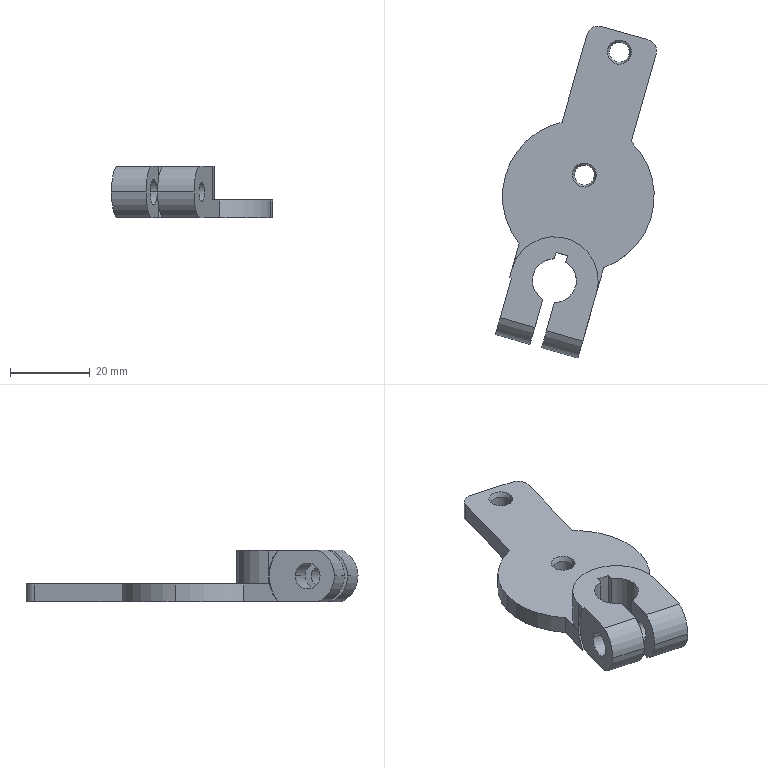Part | SolidWorks | features BaseBody 1 | 1 solid | 41 faces | box 40.361 x 83.155 x 13 mm | volume 11122 mm3 | cylinder 22 | plane 15 | cone 4 | commonest cylinder face diameters 5 x6 14 x4 11 x3 38 x3 6 x2 6.5 x2
STEP:
#1=CARTESIAN_POINT('',(388.225,129.634,54.293));
#2=VERTEX_POINT('',#1);
#3=CARTESIAN_POINT('',(393.033,128.265,54.293));
#4=VERTEX_POINT('',#3);
#5=CARTESIAN_POINT('',(390.629,128.949,54.293));
#6=DIRECTION('',(0.,0.,1.));
#7=DIRECTION('',(0.9618,-0.2738,0.));
#8=AXIS2_PLACEMENT_3D('',#5,#6,#7);
#9=CIRCLE('',#8,2.5);
#10=EDGE_CURVE('',#2,#4,#9,.T.);
#11=ORIENTED_EDGE('',*,*,#10,.F.);
#12=CARTESIAN_POINT('',(387.744,129.771,55.5));
#13=VERTEX_POINT('',#12);
#14=CARTESIAN_POINT('',(387.744,129.771,55.5));
#15=DIRECTION('',(-0.3681,0.1048,0.9239));
#16=VECTOR('',#15,1000.);
#17=LINE('',#14,#16);
#18=EDGE_CURVE('',#2,#13,#17,.T.);
#19=ORIENTED_EDGE('',*,*,#18,.T.);
#20=CARTESIAN_POINT('',(393.514,128.128,55.5));
#21=VERTEX_POINT('',#20);
#22=CARTESIAN_POINT('',(390.629,128.949,55.5));
#23=DIRECTION('',(0.,0.,1.));
#24=DIRECTION('',(0.9618,-0.2738,0.));
#25=AXIS2_PLACEMENT_3D('',#22,#23,#24);
#26=CIRCLE('',#25,3.);
#27=EDGE_CURVE('',#13,#21,#26,.T.);
#28=ORIENTED_EDGE('',*,*,#27,.T.);
#29=CARTESIAN_POINT('',(393.514,128.128,55.5));
#30=DIRECTION('',(0.3681,-0.1048,0.9239));
#31=VECTOR('',#30,1000.);
#32=LINE('',#29,#31);
#33=EDGE_CURVE('',#4,#21,#32,.T.);
#34=ORIENTED_EDGE('',*,*,#33,.F.);
#35=EDGE_LOOP('',(#11,#19,#28,#34));
#36=FACE_OUTER_BOUND('',#35,.T.);
#37=CARTESIAN_POINT('',(390.629,128.949,55.5));
#38=DIRECTION('',(0.,0.,1.));
#39=DIRECTION('',(0.9618,-0.2738,0.));
#40=AXIS2_PLACEMENT_3D('',#37,#38,#39);
#41=CONICAL_SURFACE('',#40,3.,0.3927);
#42=ADVANCED_FACE('',(#36),#41,.F.);
#43=CARTESIAN_POINT('',(388.225,129.634,51.));
#44=VERTEX_POINT('',#43);
#45=CARTESIAN_POINT('',(393.033,128.265,51.));
#46=VERTEX_POINT('',#45);
#47=CARTESIAN_POINT('',(390.629,128.949,51.));
#48=DIRECTION('',(0.,0.,1.));
#49=DIRECTION('',(0.9618,-0.2738,0.));
#50=AXIS2_PLACEMENT_3D('',#47,#48,#49);
#51=CIRCLE('',#50,2.5);
#52=EDGE_CURVE('',#44,#46,#51,.T.);
#53=ORIENTED_EDGE('',*,*,#52,.F.);
#54=CARTESIAN_POINT('',(388.225,129.634,55.5));
#55=DIRECTION('',(0.,0.,1.));
#56=VECTOR('',#55,1000.);
#57=LINE('',#54,#56);
#58=EDGE_CURVE('',#44,#2,#57,.T.);
#59=ORIENTED_EDGE('',*,*,#58,.T.);
#60=ORIENTED_EDGE('',*,*,#10,.T.);
#61=CARTESIAN_POINT('',(393.033,128.265,55.5));
#62=DIRECTION('',(0.,0.,1.));
#63=VECTOR('',#62,1000.);
#64=LINE('',#61,#63);
#65=EDGE_CURVE('',#46,#4,#64,.T.);
#66=ORIENTED_EDGE('',*,*,#65,.F.);
#67=EDGE_LOOP('',(#53,#59,#60,#66));
#68=FACE_OUTER_BOUND('',#67,.T.);
#69=CARTESIAN_POINT('',(390.629,128.949,55.5));
#70=DIRECTION('',(0.,0.,1.));
#71=DIRECTION('',(0.9618,-0.2738,0.));
#72=AXIS2_PLACEMENT_3D('',#69,#70,#71);
#73=CYLINDRICAL_SURFACE('',#72,2.5);
#74=ADVANCED_FACE('',(#68),#73,.F.);
#75=CARTESIAN_POINT('',(396.986,160.411,54.293));
#76=VERTEX_POINT('',#75);
#77=CARTESIAN_POINT('',(401.794,159.042,54.293));
#78=VERTEX_POINT('',#77);
#79=CARTESIAN_POINT('',(399.39,159.727,54.293));
#80=DIRECTION('',(0.,0.,1.));
#81=DIRECTION('',(0.9618,-0.2738,0.));
#82=AXIS2_PLACEMENT_3D('',#79,#80,#81);
#83=CIRCLE('',#82,2.5);
#84=EDGE_CURVE('',#76,#78,#83,.T.);
#85=ORIENTED_EDGE('',*,*,#84,.F.);
#86=CARTESIAN_POINT('',(396.505,160.548,55.5));
#87=VERTEX_POINT('',#86);
#88=CARTESIAN_POINT('',(396.505,160.548,55.5));
#89=DIRECTION('',(-0.3681,0.1048,0.9239));
#90=VECTOR('',#89,1000.);
#91=LINE('',#88,#90);
#92=EDGE_CURVE('',#76,#87,#91,.T.);
#93=ORIENTED_EDGE('',*,*,#92,.T.);
#94=CARTESIAN_POINT('',(402.275,158.905,55.5));
#95=VERTEX_POINT('',#94);
#96=CARTESIAN_POINT('',(399.39,159.727,55.5));
#97=DIRECTION('',(0.,0.,1.));
#98=DIRECTION('',(0.9618,-0.2738,0.));
#99=AXIS2_PLACEMENT_3D('',#96,#97,#98);
#100=CIRCLE('',#99,3.);
#101=EDGE_CURVE('',#87,#95,#100,.T.);
#102=ORIENTED_EDGE('',*,*,#101,.T.);
#103=CARTESIAN_POINT('',(402.275,158.905,55.5));
#104=DIRECTION('',(0.3681,-0.1048,0.9239));
#105=VECTOR('',#104,1000.);
#106=LINE('',#103,#105);
#107=EDGE_CURVE('',#78,#95,#106,.T.);
#108=ORIENTED_EDGE('',*,*,#107,.F.);
#109=EDGE_LOOP('',(#85,#93,#102,#108));
#110=FACE_OUTER_BOUND('',#109,.T.);
#111=CARTESIAN_POINT('',(399.39,159.727,55.5));
#112=DIRECTION('',(0.,0.,1.));
#113=DIRECTION('',(0.9618,-0.2738,0.));
#114=AXIS2_PLACEMENT_3D('',#111,#112,#113);
#115=CONICAL_SURFACE('',#114,3.,0.3927);
#116=ADVANCED_FACE('',(#110),#115,.F.);
#117=CARTESIAN_POINT('',(396.986,160.411,51.));
#118=VERTEX_POINT('',#117);
#119=CARTESIAN_POINT('',(401.794,159.042,51.));
#120=VERTEX_POINT('',#119);
#121=CARTESIAN_POINT('',(399.39,159.727,51.));
#122=DIRECTION('',(0.,0.,1.));
#123=DIRECTION('',(0.9618,-0.2738,0.));
#124=AXIS2_PLACEMENT_3D('',#121,#122,#123);
#125=CIRCLE('',#124,2.5);
#126=EDGE_CURVE('',#118,#120,#125,.T.);
#127=ORIENTED_EDGE('',*,*,#126,.F.);
#128=CARTESIAN_POINT('',(396.986,160.411,55.5));
#129=DIRECTION('',(0.,0.,1.));
#130=VECTOR('',#129,1000.);
#131=LINE('',#128,#130);
#132=EDGE_CURVE('',#118,#76,#131,.T.);
#133=ORIENTED_EDGE('',*,*,#132,.T.);
#134=ORIENTED_EDGE('',*,*,#84,.T.);
#135=CARTESIAN_POINT('',(401.794,159.042,55.5));
#136=DIRECTION('',(0.,0.,1.));
#137=VECTOR('',#136,1000.);
#138=LINE('',#135,#137);
#139=EDGE_CURVE('',#120,#78,#138,.T.);
#140=ORIENTED_EDGE('',*,*,#139,.F.);
#141=EDGE_LOOP('',(#127,#133,#134,#140));
#142=FACE_OUTER_BOUND('',#141,.T.);
#143=CARTESIAN_POINT('',(399.39,159.727,55.5));
#144=DIRECTION('',(0.,0.,1.));
#145=DIRECTION('',(0.9618,-0.2738,0.));
#146=AXIS2_PLACEMENT_3D('',#143,#144,#145);
#147=CYLINDRICAL_SURFACE('',#146,2.5);
#148=ADVANCED_FACE('',(#142),#147,.F.);
#149=CARTESIAN_POINT('',(389.025,83.138,57.5));
#150=VERTEX_POINT('',#149);
#151=CARTESIAN_POINT('',(390.231,87.372,51.));
#152=VERTEX_POINT('',#151);
#153=CARTESIAN_POINT('',(390.942,89.87,57.5));
#154=DIRECTION('',(0.9618,-0.2738,0.));
#155=DIRECTION('',(-0.2738,-0.9618,0.));
#156=AXIS2_PLACEMENT_3D('',#153,#154,#155);
#157=CIRCLE('',#156,7.);
#158=EDGE_CURVE('',#150,#152,#157,.T.);
#159=ORIENTED_EDGE('',*,*,#158,.F.);
#160=CARTESIAN_POINT('',(379.888,85.739,57.5));
#161=VERTEX_POINT('',#160);
#162=CARTESIAN_POINT('',(396.72,80.948,57.5));
#163=DIRECTION('',(-0.9618,0.2738,0.));
#164=VECTOR('',#163,1000.);
#165=LINE('',#162,#164);
#166=EDGE_CURVE('',#150,#161,#165,.T.);
#167=ORIENTED_EDGE('',*,*,#166,.T.);
#168=CARTESIAN_POINT('',(381.094,89.973,51.));
#169=VERTEX_POINT('',#168);
#170=CARTESIAN_POINT('',(381.805,92.471,57.5));
#171=DIRECTION('',(-0.9618,0.2738,0.));
#172=DIRECTION('',(0.2738,0.9618,0.));
#173=AXIS2_PLACEMENT_3D('',#170,#171,#172);
#174=CIRCLE('',#173,7.);
#175=EDGE_CURVE('',#169,#161,#174,.T.);
#176=ORIENTED_EDGE('',*,*,#175,.F.);
#177=CARTESIAN_POINT('',(397.925,85.181,51.));
#178=DIRECTION('',(-0.9618,0.2738,0.));
#179=VECTOR('',#178,1000.);
#180=LINE('',#177,#179);
#181=EDGE_CURVE('',#152,#169,#180,.T.);
#182=ORIENTED_EDGE('',*,*,#181,.F.);
#183=EDGE_LOOP('',(#159,#167,#176,#182));
#184=FACE_OUTER_BOUND('',#183,.T.);
#185=CARTESIAN_POINT('',(398.636,87.68,57.5));
#186=DIRECTION('',(-0.9618,0.2738,0.));
#187=DIRECTION('',(-0.2738,-0.9618,0.));
#188=AXIS2_PLACEMENT_3D('',#185,#186,#187);
#189=CYLINDRICAL_SURFACE('',#188,7.);
#190=ADVANCED_FACE('',(#184),#189,.T.);
#191=CARTESIAN_POINT('',(377.003,86.56,57.5));
#192=VERTEX_POINT('',#191);
#193=CARTESIAN_POINT('',(378.208,90.794,51.));
#194=VERTEX_POINT('',#193);
#195=CARTESIAN_POINT('',(378.919,93.293,57.5));
#196=DIRECTION('',(0.9618,-0.2738,0.));
#197=DIRECTION('',(-0.2738,-0.9618,0.));
#198=AXIS2_PLACEMENT_3D('',#195,#196,#197);
#199=CIRCLE('',#198,7.);
#200=EDGE_CURVE('',#192,#194,#199,.T.);
#201=ORIENTED_EDGE('',*,*,#200,.F.);
#202=CARTESIAN_POINT('',(368.347,89.024,57.5));
#203=VERTEX_POINT('',#202);
#204=CARTESIAN_POINT('',(396.72,80.948,57.5));
#205=DIRECTION('',(-0.9618,0.2738,0.));
#206=VECTOR('',#205,1000.);
#207=LINE('',#204,#206);
#208=EDGE_CURVE('',#192,#203,#207,.T.);
#209=ORIENTED_EDGE('',*,*,#208,.T.);
#210=CARTESIAN_POINT('',(369.552,93.258,51.));
#211=VERTEX_POINT('',#210);
#212=CARTESIAN_POINT('',(370.263,95.757,57.5));
#213=DIRECTION('',(0.9618,-0.2738,0.));
#214=DIRECTION('',(-0.2738,-0.9618,0.));
#215=AXIS2_PLACEMENT_3D('',#212,#213,#214);
#216=CIRCLE('',#215,7.);
#217=EDGE_CURVE('',#203,#211,#216,.T.);
#218=ORIENTED_EDGE('',*,*,#217,.T.);
#219=CARTESIAN_POINT('',(397.925,85.181,51.));
#220=DIRECTION('',(-0.9618,0.2738,0.));
#221=VECTOR('',#220,1000.);
#222=LINE('',#219,#221);
#223=EDGE_CURVE('',#194,#211,#222,.T.);
#224=ORIENTED_EDGE('',*,*,#223,.F.);
#225=EDGE_LOOP('',(#201,#209,#218,#224));
#226=FACE_OUTER_BOUND('',#225,.T.);
#227=CARTESIAN_POINT('',(398.636,87.68,57.5));
#228=DIRECTION('',(-0.9618,0.2738,0.));
#229=DIRECTION('',(-0.2738,-0.9618,0.));
#230=AXIS2_PLACEMENT_3D('',#227,#228,#229);
#231=CYLINDRICAL_SURFACE('',#230,7.);
#232=ADVANCED_FACE('',(#226),#231,.T.);
#233=CARTESIAN_POINT('',(378.03,90.167,57.5));
#234=VERTEX_POINT('',#233);
#235=CARTESIAN_POINT('',(379.809,96.419,57.5));
#236=VERTEX_POINT('',#235);
#237=CARTESIAN_POINT('',(378.919,93.293,57.5));
#238=DIRECTION('',(0.9618,-0.2738,0.));
#239=DIRECTION('',(-0.2738,-0.9618,0.));
#240=AXIS2_PLACEMENT_3D('',#237,#238,#239);
#241=CIRCLE('',#240,3.25);
#242=EDGE_CURVE('',#234,#236,#241,.T.);
#243=ORIENTED_EDGE('',*,*,#242,.T.);
#244=CARTESIAN_POINT('',(371.153,98.883,57.5));
#245=VERTEX_POINT('',#244);
#246=CARTESIAN_POINT('',(399.527,90.806,57.5));
#247=DIRECTION('',(-0.9618,0.2738,0.));
#248=VECTOR('',#247,1000.);
#249=LINE('',#246,#248);
#250=EDGE_CURVE('',#236,#245,#249,.T.);
#251=ORIENTED_EDGE('',*,*,#250,.T.);
#252=CARTESIAN_POINT('',(369.374,92.631,57.5));
#253=VERTEX_POINT('',#252);
#254=CARTESIAN_POINT('',(370.263,95.757,57.5));
#255=DIRECTION('',(-0.9618,0.2738,0.));
#256=DIRECTION('',(-0.2738,-0.9618,0.));
#257=AXIS2_PLACEMENT_3D('',#254,#255,#256);
#258=CIRCLE('',#257,3.25);
#259=EDGE_CURVE('',#245,#253,#258,.T.);
#260=ORIENTED_EDGE('',*,*,#259,.T.);
#261=CARTESIAN_POINT('',(397.747,84.554,57.5));
#262=DIRECTION('',(-0.9618,0.2738,0.));
#263=VECTOR('',#262,1000.);
#264=LINE('',#261,#263);
#265=EDGE_CURVE('',#234,#253,#264,.T.);
#266=ORIENTED_EDGE('',*,*,#265,.F.);
#267=EDGE_LOOP('',(#243,#251,#260,#266));
#268=FACE_OUTER_BOUND('',#267,.T.);
#269=CARTESIAN_POINT('',(398.637,87.68,57.5));
#270=DIRECTION('',(-0.9618,0.2738,0.));
#271=DIRECTION('',(-0.2738,-0.9618,0.));
#272=AXIS2_PLACEMENT_3D('',#269,#270,#271);
#273=CYLINDRICAL_SURFACE('',#272,3.25);
#274=ADVANCED_FACE('',(#268),#273,.F.);
#275=CARTESIAN_POINT('',(390.942,89.87,55.));
#276=VERTEX_POINT('',#275);
#277=CARTESIAN_POINT('',(390.942,89.87,60.));
#278=VERTEX_POINT('',#277);
#279=CARTESIAN_POINT('',(390.942,89.87,57.5));
#280=DIRECTION('',(-0.9618,0.2738,0.));
#281=DIRECTION('',(-0.2738,-0.9618,0.));
#282=AXIS2_PLACEMENT_3D('',#279,#280,#281);
#283=CIRCLE('',#282,2.5);
#284=EDGE_CURVE('',#276,#278,#283,.T.);
#285=ORIENTED_EDGE('',*,*,#284,.F.);
#286=CARTESIAN_POINT('',(381.805,92.471,55.));
#287=VERTEX_POINT('',#286);
#288=CARTESIAN_POINT('',(370.263,95.757,55.));
#289=DIRECTION('',(-0.9618,0.2738,0.));
#290=VECTOR('',#289,1000.);
#291=LINE('',#288,#290);
#292=EDGE_CURVE('',#276,#287,#291,.T.);
#293=ORIENTED_EDGE('',*,*,#292,.T.);
#294=CARTESIAN_POINT('',(381.805,92.471,60.));
#295=VERTEX_POINT('',#294);
#296=CARTESIAN_POINT('',(381.805,92.471,57.5));
#297=DIRECTION('',(0.9618,-0.2738,0.));
#298=DIRECTION('',(0.2738,0.9618,0.));
#299=AXIS2_PLACEMENT_3D('',#296,#297,#298);
#300=CIRCLE('',#299,2.5);
#301=EDGE_CURVE('',#295,#287,#300,.T.);
#302=ORIENTED_EDGE('',*,*,#301,.F.);
#303=CARTESIAN_POINT('',(370.263,95.757,60.));
#304=DIRECTION('',(-0.9618,0.2738,0.));
#305=VECTOR('',#304,1000.);
#306=LINE('',#303,#305);
#307=EDGE_CURVE('',#278,#295,#306,.T.);
#308=ORIENTED_EDGE('',*,*,#307,.F.);
#309=EDGE_LOOP('',(#285,#293,#302,#308));
#310=FACE_OUTER_BOUND('',#309,.T.);
#311=CARTESIAN_POINT('',(370.263,95.757,57.5));
#312=DIRECTION('',(-0.9618,0.2738,0.));
#313=DIRECTION('',(0.,0.,1.));
#314=AXIS2_PLACEMENT_3D('',#311,#312,#313);
#315=CYLINDRICAL_SURFACE('',#314,2.5);
#316=ADVANCED_FACE('',(#310),#315,.F.);
#317=CARTESIAN_POINT('',(377.81,104.006,64.));
#318=VERTEX_POINT('',#317);
#319=CARTESIAN_POINT('',(383.106,108.,64.));
#320=VERTEX_POINT('',#319);
#321=CARTESIAN_POINT('',(383.1,102.5,64.));
#322=DIRECTION('',(0.,0.,-1.));
#323=DIRECTION('',(0.9618,-0.2738,0.));
#324=AXIS2_PLACEMENT_3D('',#321,#322,#323);
#325=CIRCLE('',#324,5.5);
#326=EDGE_CURVE('',#318,#320,#325,.T.);
#327=ORIENTED_EDGE('',*,*,#326,.F.);
#328=CARTESIAN_POINT('',(377.81,104.006,51.));
#329=VERTEX_POINT('',#328);
#330=CARTESIAN_POINT('',(377.81,104.006,55.5));
#331=DIRECTION('',(0.,0.,-1.));
#332=VECTOR('',#331,1000.);
#333=LINE('',#330,#332);
#334=EDGE_CURVE('',#318,#329,#333,.T.);
#335=ORIENTED_EDGE('',*,*,#334,.T.);
#336=CARTESIAN_POINT('',(383.106,108.,51.));
#337=VERTEX_POINT('',#336);
#338=CARTESIAN_POINT('',(383.1,102.5,51.));
#339=DIRECTION('',(0.,0.,-1.));
#340=DIRECTION('',(0.9618,-0.2738,0.));
#341=AXIS2_PLACEMENT_3D('',#338,#339,#340);
#342=CIRCLE('',#341,5.5);
#343=EDGE_CURVE('',#329,#337,#342,.T.);
#344=ORIENTED_EDGE('',*,*,#343,.T.);
#345=CARTESIAN_POINT('',(383.106,108.,55.5));
#346=DIRECTION('',(0.,0.,-1.));
#347=VECTOR('',#346,1000.);
#348=LINE('',#345,#347);
#349=EDGE_CURVE('',#320,#337,#348,.T.);
#350=ORIENTED_EDGE('',*,*,#349,.F.);
#351=EDGE_LOOP('',(#327,#335,#344,#350));
#352=FACE_OUTER_BOUND('',#351,.T.);
#353=CARTESIAN_POINT('',(383.1,102.5,55.5));
#354=DIRECTION('',(0.,0.,-1.));
#355=DIRECTION('',(-0.9618,0.2738,0.));
#356=AXIS2_PLACEMENT_3D('',#353,#354,#355);
#357=CYLINDRICAL_SURFACE('',#356,5.5);
#358=ADVANCED_FACE('',(#352),#357,.F.);
#359=CARTESIAN_POINT('',(370.849,128.861,55.5));
#360=VERTEX_POINT('',#359);
#361=CARTESIAN_POINT('',(374.302,111.771,55.5));
#362=VERTEX_POINT('',#361);
#363=CARTESIAN_POINT('',(389.123,123.659,55.5));
#364=DIRECTION('',(0.,0.,1.));
#365=DIRECTION('',(0.9618,-0.2738,0.));
#366=AXIS2_PLACEMENT_3D('',#363,#364,#365);
#367=CIRCLE('',#366,19.);
#368=EDGE_CURVE('',#360,#362,#367,.T.);
#369=ORIENTED_EDGE('',*,*,#368,.F.);
#370=CARTESIAN_POINT('',(370.849,128.861,51.));
#371=VERTEX_POINT('',#370);
#372=CARTESIAN_POINT('',(370.849,128.861,55.5));
#373=DIRECTION('',(0.,0.,-1.));
#374=VECTOR('',#373,1000.);
#375=LINE('',#372,#374);
#376=EDGE_CURVE('',#360,#371,#375,.T.);
#377=ORIENTED_EDGE('',*,*,#376,.T.);
#378=CARTESIAN_POINT('',(374.302,111.771,51.));
#379=VERTEX_POINT('',#378);
#380=CARTESIAN_POINT('',(389.123,123.659,51.));
#381=DIRECTION('',(0.,0.,1.));
#382=DIRECTION('',(0.9618,-0.2738,0.));
#383=AXIS2_PLACEMENT_3D('',#380,#381,#382);
#384=CIRCLE('',#383,19.);
#385=EDGE_CURVE('',#371,#379,#384,.T.);
#386=ORIENTED_EDGE('',*,*,#385,.T.);
#387=CARTESIAN_POINT('',(374.302,111.771,55.5));
#388=DIRECTION('',(0.,0.,-1.));
#389=VECTOR('',#388,1000.);
#390=LINE('',#387,#389);
#391=EDGE_CURVE('',#362,#379,#390,.T.);
#392=ORIENTED_EDGE('',*,*,#391,.F.);
#393=EDGE_LOOP('',(#369,#377,#386,#392));
#394=FACE_OUTER_BOUND('',#393,.T.);
#395=CARTESIAN_POINT('',(389.123,123.659,55.5));
#396=DIRECTION('',(0.,0.,-1.));
#397=DIRECTION('',(-0.9618,0.2738,0.));
#398=AXIS2_PLACEMENT_3D('',#395,#396,#397);
#399=CYLINDRICAL_SURFACE('',#398,19.);
#400=ADVANCED_FACE('',(#394),#399,.T.);
#401=CARTESIAN_POINT('',(372.52,105.512,64.));
#402=VERTEX_POINT('',#401);
#403=CARTESIAN_POINT('',(372.52,105.512,57.5));
#404=VERTEX_POINT('',#403);
#405=CARTESIAN_POINT('',(372.52,105.512,64.));
#406=DIRECTION('',(0.,0.,-1.));
#407=VECTOR('',#406,1000.);
#408=LINE('',#405,#407);
#409=EDGE_CURVE('',#402,#404,#408,.T.);
#410=ORIENTED_EDGE('',*,*,#409,.T.);
#411=CARTESIAN_POINT('',(371.863,103.203,64.));
#412=VERTEX_POINT('',#411);
#413=CARTESIAN_POINT('',(369.782,95.894,57.5));
#414=DIRECTION('',(-0.9618,0.2738,0.));
#415=DIRECTION('',(-0.2738,-0.9618,0.));
#416=AXIS2_PLACEMENT_3D('',#413,#414,#415);
#417=CIRCLE('',#416,10.);
#418=EDGE_CURVE('',#412,#404,#417,.T.);
#419=ORIENTED_EDGE('',*,*,#418,.F.);
#420=CARTESIAN_POINT('',(372.52,105.512,64.));
#421=DIRECTION('',(-0.2738,-0.9618,0.));
#422=VECTOR('',#421,1000.);
#423=LINE('',#420,#422);
#424=EDGE_CURVE('',#402,#412,#423,.T.);
#425=ORIENTED_EDGE('',*,*,#424,.F.);
#426=EDGE_LOOP('',(#410,#419,#425));
#427=FACE_OUTER_BOUND('',#426,.T.);
#428=CARTESIAN_POINT('',(374.302,111.771,55.5));
#429=DIRECTION('',(0.9618,-0.2738,0.));
#430=DIRECTION('',(0.2738,0.9618,0.));
#431=AXIS2_PLACEMENT_3D('',#428,#429,#430);
#432=PLANE('',#431);
#433=ADVANCED_FACE('',(#427),#432,.F.);
#434=CARTESIAN_POINT('',(394.988,166.178,51.));
#435=VERTEX_POINT('',#434);
#436=CARTESIAN_POINT('',(391.281,164.114,51.));
#437=VERTEX_POINT('',#436);
#438=CARTESIAN_POINT('',(394.167,163.293,51.));
#439=DIRECTION('',(0.,0.,1.));
#440=DIRECTION('',(0.9618,-0.2738,0.));
#441=AXIS2_PLACEMENT_3D('',#438,#439,#440);
#442=CIRCLE('',#441,3.);
#443=EDGE_CURVE('',#435,#437,#442,.T.);
#444=ORIENTED_EDGE('',*,*,#443,.T.);
#445=CARTESIAN_POINT('',(391.281,164.114,55.5));
#446=VERTEX_POINT('',#445);
#447=CARTESIAN_POINT('',(391.281,164.114,55.5));
#448=DIRECTION('',(0.,0.,-1.));
#449=VECTOR('',#448,1000.);
#450=LINE('',#447,#449);
#451=EDGE_CURVE('',#446,#437,#450,.T.);
#452=ORIENTED_EDGE('',*,*,#451,.F.);
#453=CARTESIAN_POINT('',(394.988,166.178,55.5));
#454=VERTEX_POINT('',#453);
#455=CARTESIAN_POINT('',(394.167,163.293,55.5));
#456=DIRECTION('',(0.,0.,1.));
#457=DIRECTION('',(0.9618,-0.2738,0.));
#458=AXIS2_PLACEMENT_3D('',#455,#456,#457);
#459=CIRCLE('',#458,3.);
#460=EDGE_CURVE('',#454,#446,#459,.T.);
#461=ORIENTED_EDGE('',*,*,#460,.F.);
#462=CARTESIAN_POINT('',(394.988,166.178,55.5));
#463=DIRECTION('',(0.,0.,-1.));
#464=VECTOR('',#463,1000.);
#465=LINE('',#462,#464);
#466=EDGE_CURVE('',#454,#435,#465,.T.);
#467=ORIENTED_EDGE('',*,*,#466,.T.);
#468=EDGE_LOOP('',(#444,#452,#461,#467));
#469=FACE_OUTER_BOUND('',#468,.T.);
#470=CARTESIAN_POINT('',(394.167,163.293,55.5));
#471=DIRECTION('',(0.,0.,-1.));
#472=DIRECTION('',(-0.9618,0.2738,0.));
#473=AXIS2_PLACEMENT_3D('',#470,#471,#472);
#474=CYLINDRICAL_SURFACE('',#473,3.);
#475=ADVANCED_FACE('',(#469),#474,.T.);
#476=CARTESIAN_POINT('',(385.048,142.217,51.));
#477=VERTEX_POINT('',#476);
#478=CARTESIAN_POINT('',(391.281,164.114,51.));
#479=DIRECTION('',(-0.2738,-0.9618,0.));
#480=VECTOR('',#479,1000.);
#481=LINE('',#478,#480);
#482=EDGE_CURVE('',#437,#477,#481,.T.);
#483=ORIENTED_EDGE('',*,*,#482,.T.);
#484=CARTESIAN_POINT('',(385.048,142.217,55.5));
#485=VERTEX_POINT('',#484);
#486=CARTESIAN_POINT('',(385.048,142.217,55.5));
#487=DIRECTION('',(0.,0.,-1.));
#488=VECTOR('',#487,1000.);
#489=LINE('',#486,#488);
#490=EDGE_CURVE('',#485,#477,#489,.T.);
#491=ORIENTED_EDGE('',*,*,#490,.F.);
#492=CARTESIAN_POINT('',(391.281,164.114,55.5));
#493=DIRECTION('',(-0.2738,-0.9618,0.));
#494=VECTOR('',#493,1000.);
#495=LINE('',#492,#494);
#496=EDGE_CURVE('',#446,#485,#495,.T.);
#497=ORIENTED_EDGE('',*,*,#496,.F.);
#498=ORIENTED_EDGE('',*,*,#451,.T.);
#499=EDGE_LOOP('',(#483,#491,#497,#498));
#500=FACE_OUTER_BOUND('',#499,.T.);
#501=CARTESIAN_POINT('',(391.281,164.114,55.5));
#502=DIRECTION('',(0.9618,-0.2738,0.));
#503=DIRECTION('',(0.2738,0.9618,0.));
#504=AXIS2_PLACEMENT_3D('',#501,#502,#503);
#505=PLANE('',#504);
#506=ADVANCED_FACE('',(#500),#505,.F.);
#507=ORIENTED_EDGE('',*,*,#376,.F.);
#508=CARTESIAN_POINT('',(389.123,123.659,55.5));
#509=DIRECTION('',(0.,0.,1.));
#510=DIRECTION('',(0.9618,-0.2738,0.));
#511=AXIS2_PLACEMENT_3D('',#508,#509,#510);
#512=CIRCLE('',#511,19.);
#513=EDGE_CURVE('',#485,#360,#512,.T.);
#514=ORIENTED_EDGE('',*,*,#513,.F.);
#515=ORIENTED_EDGE('',*,*,#490,.T.);
#516=CARTESIAN_POINT('',(389.123,123.659,51.));
#517=DIRECTION('',(0.,0.,1.));
#518=DIRECTION('',(0.9618,-0.2738,0.));
#519=AXIS2_PLACEMENT_3D('',#516,#517,#518);
#520=CIRCLE('',#519,19.);
#521=EDGE_CURVE('',#477,#371,#520,.T.);
#522=ORIENTED_EDGE('',*,*,#521,.T.);
#523=EDGE_LOOP('',(#507,#514,#515,#522));
#524=FACE_OUTER_BOUND('',#523,.T.);
#525=CARTESIAN_POINT('',(389.123,123.659,55.5));
#526=DIRECTION('',(0.,0.,-1.));
#527=DIRECTION('',(-0.9618,0.2738,0.));
#528=AXIS2_PLACEMENT_3D('',#525,#526,#527);
#529=CYLINDRICAL_SURFACE('',#528,19.);
#530=ADVANCED_FACE('',(#524),#529,.T.);
#531=CARTESIAN_POINT('',(371.863,103.203,51.));
#532=VERTEX_POINT('',#531);
#533=CARTESIAN_POINT('',(374.302,111.771,51.));
#534=DIRECTION('',(-0.2738,-0.9618,0.));
#535=VECTOR('',#534,1000.);
#536=LINE('',#533,#535);
#537=EDGE_CURVE('',#379,#532,#536,.T.);
#538=ORIENTED_EDGE('',*,*,#537,.T.);
#539=CARTESIAN_POINT('',(369.782,95.894,57.5));
#540=DIRECTION('',(-0.9618,0.2738,0.));
#541=DIRECTION('',(-0.2738,-0.9618,0.));
#542=AXIS2_PLACEMENT_3D('',#539,#540,#541);
#543=CIRCLE('',#542,10.);
#544=EDGE_CURVE('',#404,#532,#543,.T.);
#545=ORIENTED_EDGE('',*,*,#544,.F.);
#546=CARTESIAN_POINT('',(372.52,105.512,55.5));
#547=VERTEX_POINT('',#546);
#548=CARTESIAN_POINT('',(372.52,105.512,64.));
#549=DIRECTION('',(0.,0.,-1.));
#550=VECTOR('',#549,1000.);
#551=LINE('',#548,#550);
#552=EDGE_CURVE('',#404,#547,#551,.T.);
#553=ORIENTED_EDGE('',*,*,#552,.T.);
#554=CARTESIAN_POINT('',(374.302,111.771,55.5));
#555=DIRECTION('',(-0.2738,-0.9618,0.));
#556=VECTOR('',#555,1000.);
#557=LINE('',#554,#556);
#558=EDGE_CURVE('',#362,#547,#557,.T.);
#559=ORIENTED_EDGE('',*,*,#558,.F.);
#560=ORIENTED_EDGE('',*,*,#391,.T.);
#561=EDGE_LOOP('',(#538,#545,#553,#559,#560));
#562=FACE_OUTER_BOUND('',#561,.T.);
#563=CARTESIAN_POINT('',(374.302,111.771,55.5));
#564=DIRECTION('',(0.9618,-0.2738,0.));
#565=DIRECTION('',(0.2738,0.9618,0.));
#566=AXIS2_PLACEMENT_3D('',#563,#564,#565);
#567=PLANE('',#566);
#568=ADVANCED_FACE('',(#562),#567,.F.);
#569=ORIENTED_EDGE('',*,*,#242,.F.);
#570=CARTESIAN_POINT('',(378.919,93.293,57.5));
#571=DIRECTION('',(0.9618,-0.2738,0.));
#572=DIRECTION('',(-0.2738,-0.9618,0.));
#573=AXIS2_PLACEMENT_3D('',#570,#571,#572);
#574=CIRCLE('',#573,3.25);
#575=EDGE_CURVE('',#236,#234,#574,.T.);
#576=ORIENTED_EDGE('',*,*,#575,.F.);
#577=EDGE_LOOP('',(#569,#576));
#578=FACE_BOUND('',#577,.T.);
#579=CARTESIAN_POINT('',(378.208,90.794,64.));
#580=VERTEX_POINT('',#579);
#581=CARTESIAN_POINT('',(380.209,97.821,64.));
#582=VERTEX_POINT('',#581);
#583=CARTESIAN_POINT('',(377.003,86.56,64.));
#584=DIRECTION('',(0.2738,0.9618,0.));
#585=VECTOR('',#584,1000.);
#586=LINE('',#583,#585);
#587=EDGE_CURVE('',#580,#582,#586,.T.);
#588=ORIENTED_EDGE('',*,*,#587,.F.);
#589=CARTESIAN_POINT('',(378.919,93.293,57.5));
#590=DIRECTION('',(0.9618,-0.2738,0.));
#591=DIRECTION('',(-0.2738,-0.9618,0.));
#592=AXIS2_PLACEMENT_3D('',#589,#590,#591);
#593=CIRCLE('',#592,7.);
#594=EDGE_CURVE('',#580,#192,#593,.T.);
#595=ORIENTED_EDGE('',*,*,#594,.T.);
#596=ORIENTED_EDGE('',*,*,#200,.T.);
#597=CARTESIAN_POINT('',(380.209,97.821,51.));
#598=VERTEX_POINT('',#597);
#599=CARTESIAN_POINT('',(380.209,97.821,51.));
#600=DIRECTION('',(0.2738,0.9618,0.));
#601=VECTOR('',#600,1000.);
#602=LINE('',#599,#601);
#603=EDGE_CURVE('',#194,#598,#602,.T.);
#604=ORIENTED_EDGE('',*,*,#603,.T.);
#605=CARTESIAN_POINT('',(380.209,97.821,55.5));
#606=DIRECTION('',(0.,0.,-1.));
#607=VECTOR('',#606,1000.);
#608=LINE('',#605,#607);
#609=EDGE_CURVE('',#582,#598,#608,.T.);
#610=ORIENTED_EDGE('',*,*,#609,.F.);
#611=EDGE_LOOP('',(#588,#595,#596,#604,#610));
#612=FACE_OUTER_BOUND('',#611,.T.);
#613=CARTESIAN_POINT('',(380.209,97.821,55.5));
#614=DIRECTION('',(-0.9618,0.2738,0.));
#615=DIRECTION('',(-0.2738,-0.9618,0.));
#616=AXIS2_PLACEMENT_3D('',#613,#614,#615);
#617=PLANE('',#616);
#618=ADVANCED_FACE('',(#578,#612),#617,.F.);
#619=ORIENTED_EDGE('',*,*,#334,.F.);
#620=CARTESIAN_POINT('',(383.1,102.5,64.));
#621=DIRECTION('',(0.,0.,-1.));
#622=DIRECTION('',(0.9618,-0.2738,0.));
#623=AXIS2_PLACEMENT_3D('',#620,#621,#622);
#624=CIRCLE('',#623,5.5);
#625=EDGE_CURVE('',#582,#318,#624,.T.);
#626=ORIENTED_EDGE('',*,*,#625,.F.);
#627=ORIENTED_EDGE('',*,*,#609,.T.);
#628=CARTESIAN_POINT('',(383.1,102.5,51.));
#629=DIRECTION('',(0.,0.,-1.));
#630=DIRECTION('',(0.9618,-0.2738,0.));
#631=AXIS2_PLACEMENT_3D('',#628,#629,#630);
#632=CIRCLE('',#631,5.5);
#633=EDGE_CURVE('',#598,#329,#632,.T.);
#634=ORIENTED_EDGE('',*,*,#633,.T.);
#635=EDGE_LOOP('',(#619,#626,#627,#634));
#636=FACE_OUTER_BOUND('',#635,.T.);
#637=CARTESIAN_POINT('',(383.1,102.5,55.5));
#638=DIRECTION('',(0.,0.,-1.));
#639=DIRECTION('',(-0.9618,0.2738,0.));
#640=AXIS2_PLACEMENT_3D('',#637,#638,#639);
#641=CYLINDRICAL_SURFACE('',#640,5.5);
#642=ADVANCED_FACE('',(#636),#641,.F.);
#643=CARTESIAN_POINT('',(383.546,109.547,51.));
#644=VERTEX_POINT('',#643);
#645=CARTESIAN_POINT('',(383.546,109.547,51.));
#646=DIRECTION('',(0.2738,0.9618,0.));
#647=VECTOR('',#646,1000.);
#648=LINE('',#645,#647);
#649=EDGE_CURVE('',#337,#644,#648,.T.);
#650=ORIENTED_EDGE('',*,*,#649,.T.);
#651=CARTESIAN_POINT('',(383.546,109.547,64.));
#652=VERTEX_POINT('',#651);
#653=CARTESIAN_POINT('',(383.546,109.547,55.5));
#654=DIRECTION('',(0.,0.,-1.));
#655=VECTOR('',#654,1000.);
#656=LINE('',#653,#655);
#657=EDGE_CURVE('',#652,#644,#656,.T.);
#658=ORIENTED_EDGE('',*,*,#657,.F.);
#659=CARTESIAN_POINT('',(383.106,108.,64.));
#660=DIRECTION('',(0.2738,0.9618,0.));
#661=VECTOR('',#660,1000.);
#662=LINE('',#659,#661);
#663=EDGE_CURVE('',#320,#652,#662,.T.);
#664=ORIENTED_EDGE('',*,*,#663,.F.);
#665=ORIENTED_EDGE('',*,*,#349,.T.);
#666=EDGE_LOOP('',(#650,#658,#664,#665));
#667=FACE_OUTER_BOUND('',#666,.T.);
#668=CARTESIAN_POINT('',(383.546,109.547,55.5));
#669=DIRECTION('',(-0.9618,0.2738,0.));
#670=DIRECTION('',(-0.2738,-0.9618,0.));
#671=AXIS2_PLACEMENT_3D('',#668,#669,#670);
#672=PLANE('',#671);
#673=ADVANCED_FACE('',(#667),#672,.F.);
#674=CARTESIAN_POINT('',(386.432,108.726,51.));
#675=VERTEX_POINT('',#674);
#676=CARTESIAN_POINT('',(383.546,109.547,51.));
#677=DIRECTION('',(0.9618,-0.2738,0.));
#678=VECTOR('',#677,1000.);
#679=LINE('',#676,#678);
#680=EDGE_CURVE('',#644,#675,#679,.T.);
#681=ORIENTED_EDGE('',*,*,#680,.T.);
#682=CARTESIAN_POINT('',(386.432,108.726,64.));
#683=VERTEX_POINT('',#682);
#684=CARTESIAN_POINT('',(386.432,108.726,55.5));
#685=DIRECTION('',(0.,0.,-1.));
#686=VECTOR('',#685,1000.);
#687=LINE('',#684,#686);
#688=EDGE_CURVE('',#683,#675,#687,.T.);
#689=ORIENTED_EDGE('',*,*,#688,.F.);
#690=CARTESIAN_POINT('',(383.546,109.547,64.));
#691=DIRECTION('',(0.9618,-0.2738,0.));
#692=VECTOR('',#691,1000.);
#693=LINE('',#690,#692);
#694=EDGE_CURVE('',#652,#683,#693,.T.);
#695=ORIENTED_EDGE('',*,*,#694,.F.);
#696=ORIENTED_EDGE('',*,*,#657,.T.);
#697=EDGE_LOOP('',(#681,#689,#695,#696));
#698=FACE_OUTER_BOUND('',#697,.T.);
#699=CARTESIAN_POINT('',(383.546,109.547,55.5));
#700=DIRECTION('',(0.2738,0.9618,0.));
#701=DIRECTION('',(0.,0.,1.));
#702=AXIS2_PLACEMENT_3D('',#699,#700,#701);
#703=PLANE('',#702);
#704=ADVANCED_FACE('',(#698),#703,.F.);
#705=CARTESIAN_POINT('',(385.991,107.179,51.));
#706=VERTEX_POINT('',#705);
#707=CARTESIAN_POINT('',(386.432,108.726,51.));
#708=DIRECTION('',(-0.2738,-0.9618,0.));
#709=VECTOR('',#708,1000.);
#710=LINE('',#707,#709);
#711=EDGE_CURVE('',#675,#706,#710,.T.);
#712=ORIENTED_EDGE('',*,*,#711,.T.);
#713=CARTESIAN_POINT('',(385.991,107.179,64.));
#714=VERTEX_POINT('',#713);
#715=CARTESIAN_POINT('',(385.991,107.179,55.5));
#716=DIRECTION('',(0.,0.,-1.));
#717=VECTOR('',#716,1000.);
#718=LINE('',#715,#717);
#719=EDGE_CURVE('',#714,#706,#718,.T.);
#720=ORIENTED_EDGE('',*,*,#719,.F.);
#721=CARTESIAN_POINT('',(386.432,108.726,64.));
#722=DIRECTION('',(-0.2738,-0.9618,0.));
#723=VECTOR('',#722,1000.);
#724=LINE('',#721,#723);
#725=EDGE_CURVE('',#683,#714,#724,.T.);
#726=ORIENTED_EDGE('',*,*,#725,.F.);
#727=ORIENTED_EDGE('',*,*,#688,.T.);
#728=EDGE_LOOP('',(#712,#720,#726,#727));
#729=FACE_OUTER_BOUND('',#728,.T.);
#730=CARTESIAN_POINT('',(386.432,108.726,55.5));
#731=DIRECTION('',(0.9618,-0.2738,0.));
#732=DIRECTION('',(0.2738,0.9618,0.));
#733=AXIS2_PLACEMENT_3D('',#730,#731,#732);
#734=PLANE('',#733);
#735=ADVANCED_FACE('',(#729),#734,.F.);
#736=CARTESIAN_POINT('',(383.094,97.,51.));
#737=VERTEX_POINT('',#736);
#738=CARTESIAN_POINT('',(383.1,102.5,51.));
#739=DIRECTION('',(0.,0.,-1.));
#740=DIRECTION('',(0.9618,-0.2738,0.));
#741=AXIS2_PLACEMENT_3D('',#738,#739,#740);
#742=CIRCLE('',#741,5.5);
#743=EDGE_CURVE('',#706,#737,#742,.T.);
#744=ORIENTED_EDGE('',*,*,#743,.T.);
#745=CARTESIAN_POINT('',(383.094,97.,64.));
#746=VERTEX_POINT('',#745);
#747=CARTESIAN_POINT('',(383.094,97.,55.5));
#748=DIRECTION('',(0.,0.,-1.));
#749=VECTOR('',#748,1000.);
#750=LINE('',#747,#749);
#751=EDGE_CURVE('',#746,#737,#750,.T.);
#752=ORIENTED_EDGE('',*,*,#751,.F.);
#753=CARTESIAN_POINT('',(383.1,102.5,64.));
#754=DIRECTION('',(0.,0.,-1.));
#755=DIRECTION('',(0.9618,-0.2738,0.));
#756=AXIS2_PLACEMENT_3D('',#753,#754,#755);
#757=CIRCLE('',#756,5.5);
#758=EDGE_CURVE('',#714,#746,#757,.T.);
#759=ORIENTED_EDGE('',*,*,#758,.F.);
#760=ORIENTED_EDGE('',*,*,#719,.T.);
#761=EDGE_LOOP('',(#744,#752,#759,#760));
#762=FACE_OUTER_BOUND('',#761,.T.);
#763=CARTESIAN_POINT('',(383.1,102.5,55.5));
#764=DIRECTION('',(0.,0.,-1.));
#765=DIRECTION('',(-0.9618,0.2738,0.));
#766=AXIS2_PLACEMENT_3D('',#763,#764,#765);
#767=CYLINDRICAL_SURFACE('',#766,5.5);
#768=ADVANCED_FACE('',(#762),#767,.F.);
#769=ORIENTED_EDGE('',*,*,#301,.T.);
#770=CARTESIAN_POINT('',(381.805,92.471,57.5));
#771=DIRECTION('',(0.9618,-0.2738,0.));
#772=DIRECTION('',(0.2738,0.9618,0.));
#773=AXIS2_PLACEMENT_3D('',#770,#771,#772);
#774=CIRCLE('',#773,2.5);
#775=EDGE_CURVE('',#287,#295,#774,.T.);
#776=ORIENTED_EDGE('',*,*,#775,.T.);
#777=EDGE_LOOP('',(#769,#776));
#778=FACE_BOUND('',#777,.T.);
#779=CARTESIAN_POINT('',(383.094,97.,51.));
#780=DIRECTION('',(-0.2738,-0.9618,0.));
#781=VECTOR('',#780,1000.);
#782=LINE('',#779,#781);
#783=EDGE_CURVE('',#737,#169,#782,.T.);
#784=ORIENTED_EDGE('',*,*,#783,.T.);
#785=ORIENTED_EDGE('',*,*,#175,.T.);
#786=CARTESIAN_POINT('',(381.094,89.973,64.));
#787=VERTEX_POINT('',#786);
#788=CARTESIAN_POINT('',(381.805,92.471,57.5));
#789=DIRECTION('',(-0.9618,0.2738,0.));
#790=DIRECTION('',(0.2738,0.9618,0.));
#791=AXIS2_PLACEMENT_3D('',#788,#789,#790);
#792=CIRCLE('',#791,7.);
#793=EDGE_CURVE('',#161,#787,#792,.T.);
#794=ORIENTED_EDGE('',*,*,#793,.T.);
#795=CARTESIAN_POINT('',(383.094,97.,64.));
#796=DIRECTION('',(-0.2738,-0.9618,0.));
#797=VECTOR('',#796,1000.);
#798=LINE('',#795,#797);
#799=EDGE_CURVE('',#746,#787,#798,.T.);
#800=ORIENTED_EDGE('',*,*,#799,.F.);
#801=ORIENTED_EDGE('',*,*,#751,.T.);
#802=EDGE_LOOP('',(#784,#785,#794,#800,#801));
#803=FACE_OUTER_BOUND('',#802,.T.);
#804=CARTESIAN_POINT('',(383.094,97.,55.5));
#805=DIRECTION('',(0.9618,-0.2738,0.));
#806=DIRECTION('',(0.2738,0.9618,0.));
#807=AXIS2_PLACEMENT_3D('',#804,#805,#806);
#808=PLANE('',#807);
#809=ADVANCED_FACE('',(#778,#803),#808,.F.);
#810=CARTESIAN_POINT('',(390.942,89.87,57.5));
#811=DIRECTION('',(-0.9618,0.2738,0.));
#812=DIRECTION('',(-0.2738,-0.9618,0.));
#813=AXIS2_PLACEMENT_3D('',#810,#811,#812);
#814=CIRCLE('',#813,2.5);
#815=EDGE_CURVE('',#278,#276,#814,.T.);
#816=ORIENTED_EDGE('',*,*,#815,.T.);
#817=ORIENTED_EDGE('',*,*,#284,.T.);
#818=EDGE_LOOP('',(#816,#817));
#819=FACE_BOUND('',#818,.T.);
#820=CARTESIAN_POINT('',(390.231,87.372,64.));
#821=VERTEX_POINT('',#820);
#822=CARTESIAN_POINT('',(393.68,99.488,64.));
#823=VERTEX_POINT('',#822);
#824=CARTESIAN_POINT('',(389.025,83.138,64.));
#825=DIRECTION('',(0.2738,0.9618,0.));
#826=VECTOR('',#825,1000.);
#827=LINE('',#824,#826);
#828=EDGE_CURVE('',#821,#823,#827,.T.);
#829=ORIENTED_EDGE('',*,*,#828,.F.);
#830=CARTESIAN_POINT('',(390.942,89.87,57.5));
#831=DIRECTION('',(0.9618,-0.2738,0.));
#832=DIRECTION('',(-0.2738,-0.9618,0.));
#833=AXIS2_PLACEMENT_3D('',#830,#831,#832);
#834=CIRCLE('',#833,7.);
#835=EDGE_CURVE('',#821,#150,#834,.T.);
#836=ORIENTED_EDGE('',*,*,#835,.T.);
#837=ORIENTED_EDGE('',*,*,#158,.T.);
#838=CARTESIAN_POINT('',(395.462,105.748,51.));
#839=VERTEX_POINT('',#838);
#840=CARTESIAN_POINT('',(395.462,105.748,51.));
#841=DIRECTION('',(0.2738,0.9618,0.));
#842=VECTOR('',#841,1000.);
#843=LINE('',#840,#842);
#844=EDGE_CURVE('',#152,#839,#843,.T.);
#845=ORIENTED_EDGE('',*,*,#844,.T.);
#846=CARTESIAN_POINT('',(395.462,105.748,55.5));
#847=VERTEX_POINT('',#846);
#848=CARTESIAN_POINT('',(395.462,105.748,55.5));
#849=DIRECTION('',(0.,0.,-1.));
#850=VECTOR('',#849,1000.);
#851=LINE('',#848,#850);
#852=EDGE_CURVE('',#847,#839,#851,.T.);
#853=ORIENTED_EDGE('',*,*,#852,.F.);
#854=CARTESIAN_POINT('',(393.68,99.488,55.5));
#855=VERTEX_POINT('',#854);
#856=CARTESIAN_POINT('',(395.462,105.748,55.5));
#857=DIRECTION('',(0.2738,0.9618,0.));
#858=VECTOR('',#857,1000.);
#859=LINE('',#856,#858);
#860=EDGE_CURVE('',#855,#847,#859,.T.);
#861=ORIENTED_EDGE('',*,*,#860,.F.);
#862=CARTESIAN_POINT('',(393.68,99.488,64.));
#863=DIRECTION('',(0.,0.,-1.));
#864=VECTOR('',#863,1000.);
#865=LINE('',#862,#864);
#866=EDGE_CURVE('',#823,#855,#865,.T.);
#867=ORIENTED_EDGE('',*,*,#866,.F.);
#868=EDGE_LOOP('',(#829,#836,#837,#845,#853,#861,#867));
#869=FACE_OUTER_BOUND('',#868,.T.);
#870=CARTESIAN_POINT('',(395.462,105.748,55.5));
#871=DIRECTION('',(-0.9618,0.2738,0.));
#872=DIRECTION('',(-0.2738,-0.9618,0.));
#873=AXIS2_PLACEMENT_3D('',#870,#871,#872);
#874=PLANE('',#873);
#875=ADVANCED_FACE('',(#819,#869),#874,.F.);
#876=CARTESIAN_POINT('',(402.361,137.289,51.));
#877=VERTEX_POINT('',#876);
#878=CARTESIAN_POINT('',(389.123,123.659,51.));
#879=DIRECTION('',(0.,0.,1.));
#880=DIRECTION('',(0.9618,-0.2738,0.));
#881=AXIS2_PLACEMENT_3D('',#878,#879,#880);
#882=CIRCLE('',#881,19.);
#883=EDGE_CURVE('',#839,#877,#882,.T.);
#884=ORIENTED_EDGE('',*,*,#883,.T.);
#885=CARTESIAN_POINT('',(402.361,137.289,55.5));
#886=VERTEX_POINT('',#885);
#887=CARTESIAN_POINT('',(402.361,137.289,55.5));
#888=DIRECTION('',(0.,0.,-1.));
#889=VECTOR('',#888,1000.);
#890=LINE('',#887,#889);
#891=EDGE_CURVE('',#886,#877,#890,.T.);
#892=ORIENTED_EDGE('',*,*,#891,.F.);
#893=CARTESIAN_POINT('',(389.123,123.659,55.5));
#894=DIRECTION('',(0.,0.,1.));
#895=DIRECTION('',(0.9618,-0.2738,0.));
#896=AXIS2_PLACEMENT_3D('',#893,#894,#895);
#897=CIRCLE('',#896,19.);
#898=EDGE_CURVE('',#847,#886,#897,.T.);
#899=ORIENTED_EDGE('',*,*,#898,.F.);
#900=ORIENTED_EDGE('',*,*,#852,.T.);
#901=EDGE_LOOP('',(#884,#892,#899,#900));
#902=FACE_OUTER_BOUND('',#901,.T.);
#903=CARTESIAN_POINT('',(389.123,123.659,55.5));
#904=DIRECTION('',(0.,0.,-1.));
#905=DIRECTION('',(-0.9618,0.2738,0.));
#906=AXIS2_PLACEMENT_3D('',#903,#904,#905);
#907=CYLINDRICAL_SURFACE('',#906,19.);
#908=ADVANCED_FACE('',(#902),#907,.T.);
#909=CARTESIAN_POINT('',(408.594,159.186,51.));
#910=VERTEX_POINT('',#909);
#911=CARTESIAN_POINT('',(408.594,159.186,51.));
#912=DIRECTION('',(0.2738,0.9618,0.));
#913=VECTOR('',#912,1000.);
#914=LINE('',#911,#913);
#915=EDGE_CURVE('',#877,#910,#914,.T.);
#916=ORIENTED_EDGE('',*,*,#915,.T.);
#917=CARTESIAN_POINT('',(408.594,159.186,55.5));
#918=VERTEX_POINT('',#917);
#919=CARTESIAN_POINT('',(408.594,159.186,55.5));
#920=DIRECTION('',(0.,0.,-1.));
#921=VECTOR('',#920,1000.);
#922=LINE('',#919,#921);
#923=EDGE_CURVE('',#918,#910,#922,.T.);
#924=ORIENTED_EDGE('',*,*,#923,.F.);
#925=CARTESIAN_POINT('',(408.594,159.186,55.5));
#926=DIRECTION('',(0.2738,0.9618,0.));
#927=VECTOR('',#926,1000.);
#928=LINE('',#925,#927);
#929=EDGE_CURVE('',#886,#918,#928,.T.);
#930=ORIENTED_EDGE('',*,*,#929,.F.);
#931=ORIENTED_EDGE('',*,*,#891,.T.);
#932=EDGE_LOOP('',(#916,#924,#930,#931));
#933=FACE_OUTER_BOUND('',#932,.T.);
#934=CARTESIAN_POINT('',(408.594,159.186,55.5));
#935=DIRECTION('',(-0.9618,0.2738,0.));
#936=DIRECTION('',(-0.2738,-0.9618,0.));
#937=AXIS2_PLACEMENT_3D('',#934,#935,#936);
#938=PLANE('',#937);
#939=ADVANCED_FACE('',(#933),#938,.F.);
#940=CARTESIAN_POINT('',(406.53,162.893,51.));
#941=VERTEX_POINT('',#940);
#942=CARTESIAN_POINT('',(405.708,160.008,51.));
#943=DIRECTION('',(0.,0.,1.));
#944=DIRECTION('',(-0.9618,0.2738,0.));
#945=AXIS2_PLACEMENT_3D('',#942,#943,#944);
#946=CIRCLE('',#945,3.);
#947=EDGE_CURVE('',#910,#941,#946,.T.);
#948=ORIENTED_EDGE('',*,*,#947,.T.);
#949=CARTESIAN_POINT('',(406.53,162.893,55.5));
#950=VERTEX_POINT('',#949);
#951=CARTESIAN_POINT('',(406.53,162.893,55.5));
#952=DIRECTION('',(0.,0.,-1.));
#953=VECTOR('',#952,1000.);
#954=LINE('',#951,#953);
#955=EDGE_CURVE('',#950,#941,#954,.T.);
#956=ORIENTED_EDGE('',*,*,#955,.F.);
#957=CARTESIAN_POINT('',(405.708,160.008,55.5));
#958=DIRECTION('',(0.,0.,1.));
#959=DIRECTION('',(-0.9618,0.2738,0.));
#960=AXIS2_PLACEMENT_3D('',#957,#958,#959);
#961=CIRCLE('',#960,3.);
#962=EDGE_CURVE('',#918,#950,#961,.T.);
#963=ORIENTED_EDGE('',*,*,#962,.F.);
#964=ORIENTED_EDGE('',*,*,#923,.T.);
#965=EDGE_LOOP('',(#948,#956,#963,#964));
#966=FACE_OUTER_BOUND('',#965,.T.);
#967=CARTESIAN_POINT('',(405.708,160.008,55.5));
#968=DIRECTION('',(0.,0.,-1.));
#969=DIRECTION('',(-0.9618,0.2738,0.));
#970=AXIS2_PLACEMENT_3D('',#967,#968,#969);
#971=CYLINDRICAL_SURFACE('',#970,3.);
#972=ADVANCED_FACE('',(#966),#971,.T.);
#973=CARTESIAN_POINT('',(394.988,166.178,51.));
#974=DIRECTION('',(-0.9618,0.2738,0.));
#975=VECTOR('',#974,1000.);
#976=LINE('',#973,#975);
#977=EDGE_CURVE('',#941,#435,#976,.T.);
#978=ORIENTED_EDGE('',*,*,#977,.T.);
#979=ORIENTED_EDGE('',*,*,#466,.F.);
#980=CARTESIAN_POINT('',(394.988,166.178,55.5));
#981=DIRECTION('',(-0.9618,0.2738,0.));
#982=VECTOR('',#981,1000.);
#983=LINE('',#980,#982);
#984=EDGE_CURVE('',#950,#454,#983,.T.);
#985=ORIENTED_EDGE('',*,*,#984,.F.);
#986=ORIENTED_EDGE('',*,*,#955,.T.);
#987=EDGE_LOOP('',(#978,#979,#985,#986));
#988=FACE_OUTER_BOUND('',#987,.T.);
#989=CARTESIAN_POINT('',(394.988,166.178,55.5));
#990=DIRECTION('',(-0.2738,-0.9618,0.));
#991=DIRECTION('',(0.,0.,-1.));
#992=AXIS2_PLACEMENT_3D('',#989,#990,#991);
#993=PLANE('',#992);
#994=ADVANCED_FACE('',(#988),#993,.F.);
#995=CARTESIAN_POINT('',(390.629,128.949,55.5));
#996=DIRECTION('',(0.,0.,1.));
#997=DIRECTION('',(0.9618,-0.2738,0.));
#998=AXIS2_PLACEMENT_3D('',#995,#996,#997);
#999=CIRCLE('',#998,3.);
#1000=EDGE_CURVE('',#21,#13,#999,.T.);
#1001=ORIENTED_EDGE('',*,*,#1000,.F.);
#1002=ORIENTED_EDGE('',*,*,#27,.F.);
#1003=EDGE_LOOP('',(#1001,#1002));
#1004=FACE_BOUND('',#1003,.T.);
#1005=CARTESIAN_POINT('',(399.39,159.727,55.5));
#1006=DIRECTION('',(0.,0.,1.));
#1007=DIRECTION('',(0.9618,-0.2738,0.));
#1008=AXIS2_PLACEMENT_3D('',#1005,#1006,#1007);
#1009=CIRCLE('',#1008,3.);
#1010=EDGE_CURVE('',#95,#87,#1009,.T.);
#1011=ORIENTED_EDGE('',*,*,#1010,.F.);
#1012=ORIENTED_EDGE('',*,*,#101,.F.);
#1013=EDGE_LOOP('',(#1011,#1012));
#1014=FACE_BOUND('',#1013,.T.);
#1015=CARTESIAN_POINT('',(383.1,102.5,55.5));
#1016=DIRECTION('',(0.,0.,1.));
#1017=DIRECTION('',(0.9618,-0.2738,0.));
#1018=AXIS2_PLACEMENT_3D('',#1015,#1016,#1017);
#1019=CIRCLE('',#1018,11.);
#1020=EDGE_CURVE('',#855,#547,#1019,.T.);
#1021=ORIENTED_EDGE('',*,*,#1020,.F.);
#1022=ORIENTED_EDGE('',*,*,#860,.T.);
#1023=ORIENTED_EDGE('',*,*,#898,.T.);
#1024=ORIENTED_EDGE('',*,*,#929,.T.);
#1025=ORIENTED_EDGE('',*,*,#962,.T.);
#1026=ORIENTED_EDGE('',*,*,#984,.T.);
#1027=ORIENTED_EDGE('',*,*,#460,.T.);
#1028=ORIENTED_EDGE('',*,*,#496,.T.);
#1029=ORIENTED_EDGE('',*,*,#513,.T.);
#1030=ORIENTED_EDGE('',*,*,#368,.T.);
#1031=ORIENTED_EDGE('',*,*,#558,.T.);
#1032=EDGE_LOOP('',(#1021,#1022,#1023,#1024,#1025,#1026,#1027,#1028,#1029,#1030,#1031));
#1033=FACE_OUTER_BOUND('',#1032,.T.);
#1034=CARTESIAN_POINT('',(394.167,163.293,55.5));
#1035=DIRECTION('',(0.,0.,1.));
#1036=DIRECTION('',(0.9618,-0.2738,0.));
#1037=AXIS2_PLACEMENT_3D('',#1034,#1035,#1036);
#1038=PLANE('',#1037);
#1039=ADVANCED_FACE('',(#1004,#1014,#1033),#1038,.T.);
#1040=CARTESIAN_POINT('',(390.629,128.949,51.));
#1041=DIRECTION('',(0.,0.,1.));
#1042=DIRECTION('',(0.9618,-0.2738,0.));
#1043=AXIS2_PLACEMENT_3D('',#1040,#1041,#1042);
#1044=CIRCLE('',#1043,2.5);
#1045=EDGE_CURVE('',#46,#44,#1044,.T.);
#1046=ORIENTED_EDGE('',*,*,#1045,.T.);
#1047=ORIENTED_EDGE('',*,*,#52,.T.);
#1048=EDGE_LOOP('',(#1046,#1047));
#1049=FACE_BOUND('',#1048,.T.);
#1050=CARTESIAN_POINT('',(399.39,159.727,51.));
#1051=DIRECTION('',(0.,0.,1.));
#1052=DIRECTION('',(0.9618,-0.2738,0.));
#1053=AXIS2_PLACEMENT_3D('',#1050,#1051,#1052);
#1054=CIRCLE('',#1053,2.5);
#1055=EDGE_CURVE('',#120,#118,#1054,.T.);
#1056=ORIENTED_EDGE('',*,*,#1055,.T.);
#1057=ORIENTED_EDGE('',*,*,#126,.T.);
#1058=EDGE_LOOP('',(#1056,#1057));
#1059=FACE_BOUND('',#1058,.T.);
#1060=ORIENTED_EDGE('',*,*,#844,.F.);
#1061=ORIENTED_EDGE('',*,*,#181,.T.);
#1062=ORIENTED_EDGE('',*,*,#783,.F.);
#1063=ORIENTED_EDGE('',*,*,#743,.F.);
#1064=ORIENTED_EDGE('',*,*,#711,.F.);
#1065=ORIENTED_EDGE('',*,*,#680,.F.);
#1066=ORIENTED_EDGE('',*,*,#649,.F.);
#1067=ORIENTED_EDGE('',*,*,#343,.F.);
#1068=ORIENTED_EDGE('',*,*,#633,.F.);
#1069=ORIENTED_EDGE('',*,*,#603,.F.);
#1070=ORIENTED_EDGE('',*,*,#223,.T.);
#1071=CARTESIAN_POINT('',(372.344,103.066,51.));
#1072=VERTEX_POINT('',#1071);
#1073=CARTESIAN_POINT('',(389.839,164.525,51.));
#1074=DIRECTION('',(-0.2738,-0.9618,0.));
#1075=VECTOR('',#1074,1000.);
#1076=LINE('',#1073,#1075);
#1077=EDGE_CURVE('',#1072,#211,#1076,.T.);
#1078=ORIENTED_EDGE('',*,*,#1077,.F.);
#1079=CARTESIAN_POINT('',(372.344,103.066,51.));
#1080=DIRECTION('',(-0.9618,0.2738,0.));
#1081=VECTOR('',#1080,1000.);
#1082=LINE('',#1079,#1081);
#1083=EDGE_CURVE('',#1072,#532,#1082,.T.);
#1084=ORIENTED_EDGE('',*,*,#1083,.T.);
#1085=ORIENTED_EDGE('',*,*,#537,.F.);
#1086=ORIENTED_EDGE('',*,*,#385,.F.);
#1087=ORIENTED_EDGE('',*,*,#521,.F.);
#1088=ORIENTED_EDGE('',*,*,#482,.F.);
#1089=ORIENTED_EDGE('',*,*,#443,.F.);
#1090=ORIENTED_EDGE('',*,*,#977,.F.);
#1091=ORIENTED_EDGE('',*,*,#947,.F.);
#1092=ORIENTED_EDGE('',*,*,#915,.F.);
#1093=ORIENTED_EDGE('',*,*,#883,.F.);
#1094=EDGE_LOOP('',(#1060,#1061,#1062,#1063,#1064,#1065,#1066,#1067,#1068,#1069,#1070,#1078,#1084,#1085,#1086,#1087,#1088,#1089,#1090,#1091,#1092,#1093));
#1095=FACE_OUTER_BOUND('',#1094,.T.);
#1096=CARTESIAN_POINT('',(394.167,163.293,51.));
#1097=DIRECTION('',(0.,0.,1.));
#1098=DIRECTION('',(0.9618,-0.2738,0.));
#1099=AXIS2_PLACEMENT_3D('',#1096,#1097,#1098);
#1100=PLANE('',#1099);
#1101=ADVANCED_FACE('',(#1049,#1059,#1095),#1100,.F.);
#1102=ORIENTED_EDGE('',*,*,#1020,.T.);
#1103=ORIENTED_EDGE('',*,*,#552,.F.);
#1104=ORIENTED_EDGE('',*,*,#409,.F.);
#1105=CARTESIAN_POINT('',(383.1,102.5,64.));
#1106=DIRECTION('',(0.,0.,1.));
#1107=DIRECTION('',(0.9618,-0.2738,0.));
#1108=AXIS2_PLACEMENT_3D('',#1105,#1106,#1107);
#1109=CIRCLE('',#1108,11.);
#1110=EDGE_CURVE('',#823,#402,#1109,.T.);
#1111=ORIENTED_EDGE('',*,*,#1110,.F.);
#1112=ORIENTED_EDGE('',*,*,#866,.T.);
#1113=EDGE_LOOP('',(#1102,#1103,#1104,#1111,#1112));
#1114=FACE_OUTER_BOUND('',#1113,.T.);
#1115=CARTESIAN_POINT('',(383.1,102.5,64.));
#1116=DIRECTION('',(0.,0.,-1.));
#1117=DIRECTION('',(-0.9618,0.2738,0.));
#1118=AXIS2_PLACEMENT_3D('',#1115,#1116,#1117);
#1119=CYLINDRICAL_SURFACE('',#1118,11.);
#1120=ADVANCED_FACE('',(#1114),#1119,.T.);
#1121=CARTESIAN_POINT('',(397.925,85.181,64.));
#1122=DIRECTION('',(-0.9618,0.2738,0.));
#1123=VECTOR('',#1122,1000.);
#1124=LINE('',#1121,#1123);
#1125=EDGE_CURVE('',#821,#787,#1124,.T.);
#1126=ORIENTED_EDGE('',*,*,#1125,.F.);
#1127=ORIENTED_EDGE('',*,*,#828,.T.);
#1128=ORIENTED_EDGE('',*,*,#1110,.T.);
#1129=ORIENTED_EDGE('',*,*,#424,.T.);
#1130=CARTESIAN_POINT('',(372.344,103.066,64.));
#1131=VERTEX_POINT('',#1130);
#1132=CARTESIAN_POINT('',(372.344,103.066,64.));
#1133=DIRECTION('',(-0.9618,0.2738,0.));
#1134=VECTOR('',#1133,1000.);
#1135=LINE('',#1132,#1134);
#1136=EDGE_CURVE('',#1131,#412,#1135,.T.);
#1137=ORIENTED_EDGE('',*,*,#1136,.F.);
#1138=CARTESIAN_POINT('',(369.552,93.258,64.));
#1139=VERTEX_POINT('',#1138);
#1140=CARTESIAN_POINT('',(373.001,105.375,64.));
#1141=DIRECTION('',(-0.2738,-0.9618,0.));
#1142=VECTOR('',#1141,1000.);
#1143=LINE('',#1140,#1142);
#1144=EDGE_CURVE('',#1131,#1139,#1143,.T.);
#1145=ORIENTED_EDGE('',*,*,#1144,.T.);
#1146=CARTESIAN_POINT('',(397.925,85.181,64.));
#1147=DIRECTION('',(-0.9618,0.2738,0.));
#1148=VECTOR('',#1147,1000.);
#1149=LINE('',#1146,#1148);
#1150=EDGE_CURVE('',#580,#1139,#1149,.T.);
#1151=ORIENTED_EDGE('',*,*,#1150,.F.);
#1152=ORIENTED_EDGE('',*,*,#587,.T.);
#1153=ORIENTED_EDGE('',*,*,#625,.T.);
#1154=ORIENTED_EDGE('',*,*,#326,.T.);
#1155=ORIENTED_EDGE('',*,*,#663,.T.);
#1156=ORIENTED_EDGE('',*,*,#694,.T.);
#1157=ORIENTED_EDGE('',*,*,#725,.T.);
#1158=ORIENTED_EDGE('',*,*,#758,.T.);
#1159=ORIENTED_EDGE('',*,*,#799,.T.);
#1160=EDGE_LOOP('',(#1126,#1127,#1128,#1129,#1137,#1145,#1151,#1152,#1153,#1154,#1155,#1156,#1157,#1158,#1159));
#1161=FACE_OUTER_BOUND('',#1160,.T.);
#1162=CARTESIAN_POINT('',(383.1,102.5,64.));
#1163=DIRECTION('',(0.,0.,1.));
#1164=DIRECTION('',(0.9618,-0.2738,0.));
#1165=AXIS2_PLACEMENT_3D('',#1162,#1163,#1164);
#1166=PLANE('',#1165);
#1167=ADVANCED_FACE('',(#1161),#1166,.T.);
#1168=CARTESIAN_POINT('',(370.263,95.757,57.5));
#1169=DIRECTION('',(-0.9618,0.2738,0.));
#1170=DIRECTION('',(-0.2738,-0.9618,0.));
#1171=AXIS2_PLACEMENT_3D('',#1168,#1169,#1170);
#1172=CIRCLE('',#1171,10.);
#1173=EDGE_CURVE('',#1131,#1072,#1172,.T.);
#1174=ORIENTED_EDGE('',*,*,#1173,.F.);
#1175=ORIENTED_EDGE('',*,*,#1136,.T.);
#1176=ORIENTED_EDGE('',*,*,#418,.T.);
#1177=ORIENTED_EDGE('',*,*,#544,.T.);
#1178=ORIENTED_EDGE('',*,*,#1083,.F.);
#1179=EDGE_LOOP('',(#1174,#1175,#1176,#1177,#1178));
#1180=FACE_OUTER_BOUND('',#1179,.T.);
#1181=CARTESIAN_POINT('',(370.263,95.757,57.5));
#1182=DIRECTION('',(-0.9618,0.2738,0.));
#1183=DIRECTION('',(-0.2738,-0.9618,0.));
#1184=AXIS2_PLACEMENT_3D('',#1181,#1182,#1183);
#1185=CYLINDRICAL_SURFACE('',#1184,10.);
#1186=ADVANCED_FACE('',(#1180),#1185,.F.);
#1187=CARTESIAN_POINT('',(370.263,95.757,57.5));
#1188=DIRECTION('',(0.9618,-0.2738,0.));
#1189=DIRECTION('',(-0.2738,-0.9618,0.));
#1190=AXIS2_PLACEMENT_3D('',#1187,#1188,#1189);
#1191=CIRCLE('',#1190,7.);
#1192=EDGE_CURVE('',#1139,#203,#1191,.T.);
#1193=ORIENTED_EDGE('',*,*,#1192,.F.);
#1194=ORIENTED_EDGE('',*,*,#1144,.F.);
#1195=ORIENTED_EDGE('',*,*,#1173,.T.);
#1196=ORIENTED_EDGE('',*,*,#1077,.T.);
#1197=ORIENTED_EDGE('',*,*,#217,.F.);
#1198=EDGE_LOOP('',(#1193,#1194,#1195,#1196,#1197));
#1199=FACE_OUTER_BOUND('',#1198,.T.);
#1200=CARTESIAN_POINT('',(370.263,95.757,57.5));
#1201=DIRECTION('',(-0.9618,0.2738,0.));
#1202=DIRECTION('',(-0.2738,-0.9618,0.));
#1203=AXIS2_PLACEMENT_3D('',#1200,#1201,#1202);
#1204=CIRCLE('',#1203,3.25);
#1205=EDGE_CURVE('',#253,#245,#1204,.T.);
#1206=ORIENTED_EDGE('',*,*,#1205,.F.);
#1207=ORIENTED_EDGE('',*,*,#259,.F.);
#1208=EDGE_LOOP('',(#1206,#1207));
#1209=FACE_BOUND('',#1208,.T.);
#1210=CARTESIAN_POINT('',(370.263,95.757,57.5));
#1211=DIRECTION('',(-0.9618,0.2738,0.));
#1212=DIRECTION('',(-0.2738,-0.9618,0.));
#1213=AXIS2_PLACEMENT_3D('',#1210,#1211,#1212);
#1214=PLANE('',#1213);
#1215=ADVANCED_FACE('',(#1199,#1209),#1214,.T.);
#1216=ORIENTED_EDGE('',*,*,#292,.F.);
#1217=ORIENTED_EDGE('',*,*,#815,.F.);
#1218=ORIENTED_EDGE('',*,*,#307,.T.);
#1219=ORIENTED_EDGE('',*,*,#775,.F.);
#1220=EDGE_LOOP('',(#1216,#1217,#1218,#1219));
#1221=FACE_OUTER_BOUND('',#1220,.T.);
#1222=CARTESIAN_POINT('',(370.263,95.757,57.5));
#1223=DIRECTION('',(-0.9618,0.2738,0.));
#1224=DIRECTION('',(0.,0.,1.));
#1225=AXIS2_PLACEMENT_3D('',#1222,#1223,#1224);
#1226=CYLINDRICAL_SURFACE('',#1225,2.5);
#1227=ADVANCED_FACE('',(#1221),#1226,.F.);
#1228=ORIENTED_EDGE('',*,*,#250,.F.);
#1229=ORIENTED_EDGE('',*,*,#575,.T.);
#1230=ORIENTED_EDGE('',*,*,#265,.T.);
#1231=ORIENTED_EDGE('',*,*,#1205,.T.);
#1232=EDGE_LOOP('',(#1228,#1229,#1230,#1231));
#1233=FACE_OUTER_BOUND('',#1232,.T.);
#1234=CARTESIAN_POINT('',(398.637,87.68,57.5));
#1235=DIRECTION('',(-0.9618,0.2738,0.));
#1236=DIRECTION('',(-0.2738,-0.9618,0.));
#1237=AXIS2_PLACEMENT_3D('',#1234,#1235,#1236);
#1238=CYLINDRICAL_SURFACE('',#1237,3.25);
#1239=ADVANCED_FACE('',(#1233),#1238,.F.);
#1240=ORIENTED_EDGE('',*,*,#208,.F.);
#1241=ORIENTED_EDGE('',*,*,#594,.F.);
#1242=ORIENTED_EDGE('',*,*,#1150,.T.);
#1243=ORIENTED_EDGE('',*,*,#1192,.T.);
#1244=EDGE_LOOP('',(#1240,#1241,#1242,#1243));
#1245=FACE_OUTER_BOUND('',#1244,.T.);
#1246=CARTESIAN_POINT('',(398.636,87.68,57.5));
#1247=DIRECTION('',(-0.9618,0.2738,0.));
#1248=DIRECTION('',(-0.2738,-0.9618,0.));
#1249=AXIS2_PLACEMENT_3D('',#1246,#1247,#1248);
#1250=CYLINDRICAL_SURFACE('',#1249,7.);
#1251=ADVANCED_FACE('',(#1245),#1250,.T.);
#1252=ORIENTED_EDGE('',*,*,#166,.F.);
#1253=ORIENTED_EDGE('',*,*,#835,.F.);
#1254=ORIENTED_EDGE('',*,*,#1125,.T.);
#1255=ORIENTED_EDGE('',*,*,#793,.F.);
#1256=EDGE_LOOP('',(#1252,#1253,#1254,#1255));
#1257=FACE_OUTER_BOUND('',#1256,.T.);
#1258=CARTESIAN_POINT('',(398.636,87.68,57.5));
#1259=DIRECTION('',(-0.9618,0.2738,0.));
#1260=DIRECTION('',(-0.2738,-0.9618,0.));
#1261=AXIS2_PLACEMENT_3D('',#1258,#1259,#1260);
#1262=CYLINDRICAL_SURFACE('',#1261,7.);
#1263=ADVANCED_FACE('',(#1257),#1262,.T.);
#1264=ORIENTED_EDGE('',*,*,#132,.F.);
#1265=ORIENTED_EDGE('',*,*,#1055,.F.);
#1266=ORIENTED_EDGE('',*,*,#139,.T.);
#1267=CARTESIAN_POINT('',(399.39,159.727,54.293));
#1268=DIRECTION('',(0.,0.,1.));
#1269=DIRECTION('',(0.9618,-0.2738,0.));
#1270=AXIS2_PLACEMENT_3D('',#1267,#1268,#1269);
#1271=CIRCLE('',#1270,2.5);
#1272=EDGE_CURVE('',#78,#76,#1271,.T.);
#1273=ORIENTED_EDGE('',*,*,#1272,.T.);
#1274=EDGE_LOOP('',(#1264,#1265,#1266,#1273));
#1275=FACE_OUTER_BOUND('',#1274,.T.);
#1276=CARTESIAN_POINT('',(399.39,159.727,55.5));
#1277=DIRECTION('',(0.,0.,1.));
#1278=DIRECTION('',(0.9618,-0.2738,0.));
#1279=AXIS2_PLACEMENT_3D('',#1276,#1277,#1278);
#1280=CYLINDRICAL_SURFACE('',#1279,2.5);
#1281=ADVANCED_FACE('',(#1275),#1280,.F.);
#1282=ORIENTED_EDGE('',*,*,#92,.F.);
#1283=ORIENTED_EDGE('',*,*,#1272,.F.);
#1284=ORIENTED_EDGE('',*,*,#107,.T.);
#1285=ORIENTED_EDGE('',*,*,#1010,.T.);
#1286=EDGE_LOOP('',(#1282,#1283,#1284,#1285));
#1287=FACE_OUTER_BOUND('',#1286,.T.);
#1288=CARTESIAN_POINT('',(399.39,159.727,55.5));
#1289=DIRECTION('',(0.,0.,1.));
#1290=DIRECTION('',(0.9618,-0.2738,0.));
#1291=AXIS2_PLACEMENT_3D('',#1288,#1289,#1290);
#1292=CONICAL_SURFACE('',#1291,3.,0.3927);
#1293=ADVANCED_FACE('',(#1287),#1292,.F.);
#1294=ORIENTED_EDGE('',*,*,#58,.F.);
#1295=ORIENTED_EDGE('',*,*,#1045,.F.);
#1296=ORIENTED_EDGE('',*,*,#65,.T.);
#1297=CARTESIAN_POINT('',(390.629,128.949,54.293));
#1298=DIRECTION('',(0.,0.,1.));
#1299=DIRECTION('',(0.9618,-0.2738,0.));
#1300=AXIS2_PLACEMENT_3D('',#1297,#1298,#1299);
#1301=CIRCLE('',#1300,2.5);
#1302=EDGE_CURVE('',#4,#2,#1301,.T.);
#1303=ORIENTED_EDGE('',*,*,#1302,.T.);
#1304=EDGE_LOOP('',(#1294,#1295,#1296,#1303));
#1305=FACE_OUTER_BOUND('',#1304,.T.);
#1306=CARTESIAN_POINT('',(390.629,128.949,55.5));
#1307=DIRECTION('',(0.,0.,1.));
#1308=DIRECTION('',(0.9618,-0.2738,0.));
#1309=AXIS2_PLACEMENT_3D('',#1306,#1307,#1308);
#1310=CYLINDRICAL_SURFACE('',#1309,2.5);
#1311=ADVANCED_FACE('',(#1305),#1310,.F.);
#1312=ORIENTED_EDGE('',*,*,#18,.F.);
#1313=ORIENTED_EDGE('',*,*,#1302,.F.);
#1314=ORIENTED_EDGE('',*,*,#33,.T.);
#1315=ORIENTED_EDGE('',*,*,#1000,.T.);
#1316=EDGE_LOOP('',(#1312,#1313,#1314,#1315));
#1317=FACE_OUTER_BOUND('',#1316,.T.);
#1318=CARTESIAN_POINT('',(390.629,128.949,55.5));
#1319=DIRECTION('',(0.,0.,1.));
#1320=DIRECTION('',(0.9618,-0.2738,0.));
#1321=AXIS2_PLACEMENT_3D('',#1318,#1319,#1320);
#1322=CONICAL_SURFACE('',#1321,3.,0.3927);
#1323=ADVANCED_FACE('',(#1317),#1322,.F.);
#1324=CLOSED_SHELL('',(#42,#74,#116,#148,#190,#232,#274,#316,#358,#400,#433,#475,#506,#530,#568,#618,#642,#673,#704,#735,#768,#809,#875,#908,#939,#972,#994,#1039,#1101,#1120,#1167,#1186,#1215,#1227,#1239,#1251,#1263,#1281,#1293,#1311,#1323));
#1325=MANIFOLD_SOLID_BREP('',#1324);
#1326=CARTESIAN_POINT('',(0.,0.,0.));
#1327=DIRECTION('',(0.,0.,1.));
#1328=DIRECTION('',(1.,0.,0.));
#1329=AXIS2_PLACEMENT_3D('',#1326,#1327,#1328);
#1330=(LENGTH_UNIT()NAMED_UNIT(*)SI_UNIT(.MILLI.,.METRE.));
#1331=UNCERTAINTY_MEASURE_WITH_UNIT(LENGTH_MEASURE(0.00001),#1330,'','');
#1332=(NAMED_UNIT(*)PLANE_ANGLE_UNIT()SI_UNIT($,.RADIAN.));
#1333=(NAMED_UNIT(*)SI_UNIT($,.STERADIAN.)SOLID_ANGLE_UNIT());
#1334=(GEOMETRIC_REPRESENTATION_CONTEXT(3)GLOBAL_UNCERTAINTY_ASSIGNED_CONTEXT((#1331))GLOBAL_UNIT_ASSIGNED_CONTEXT((#1330,#1332,#1333))REPRESENTATION_CONTEXT('',''));
#1335=ADVANCED_BREP_SHAPE_REPRESENTATION('',(#1325,#1329),#1334);